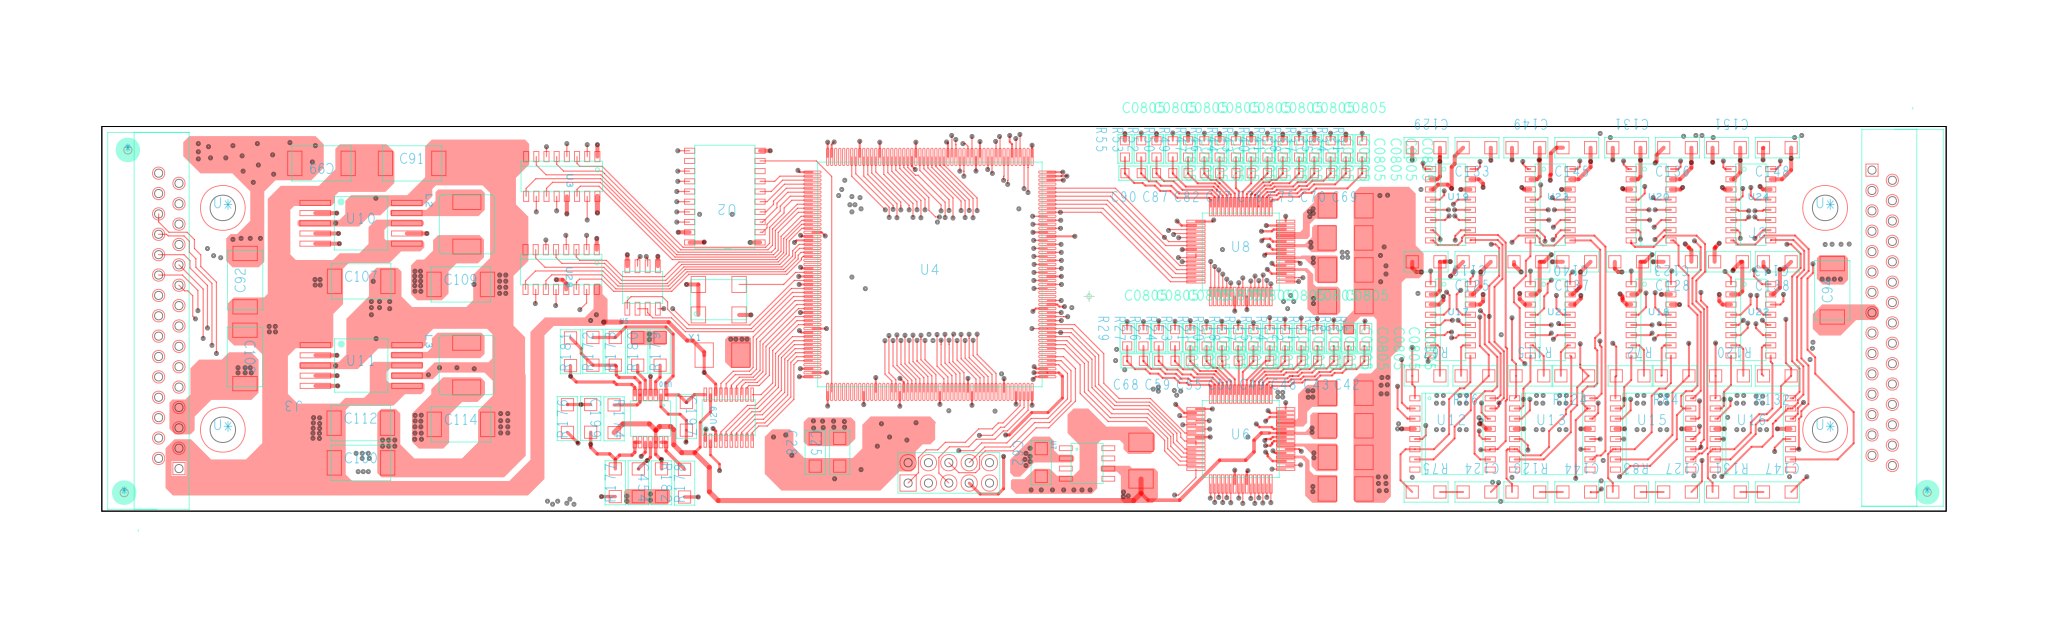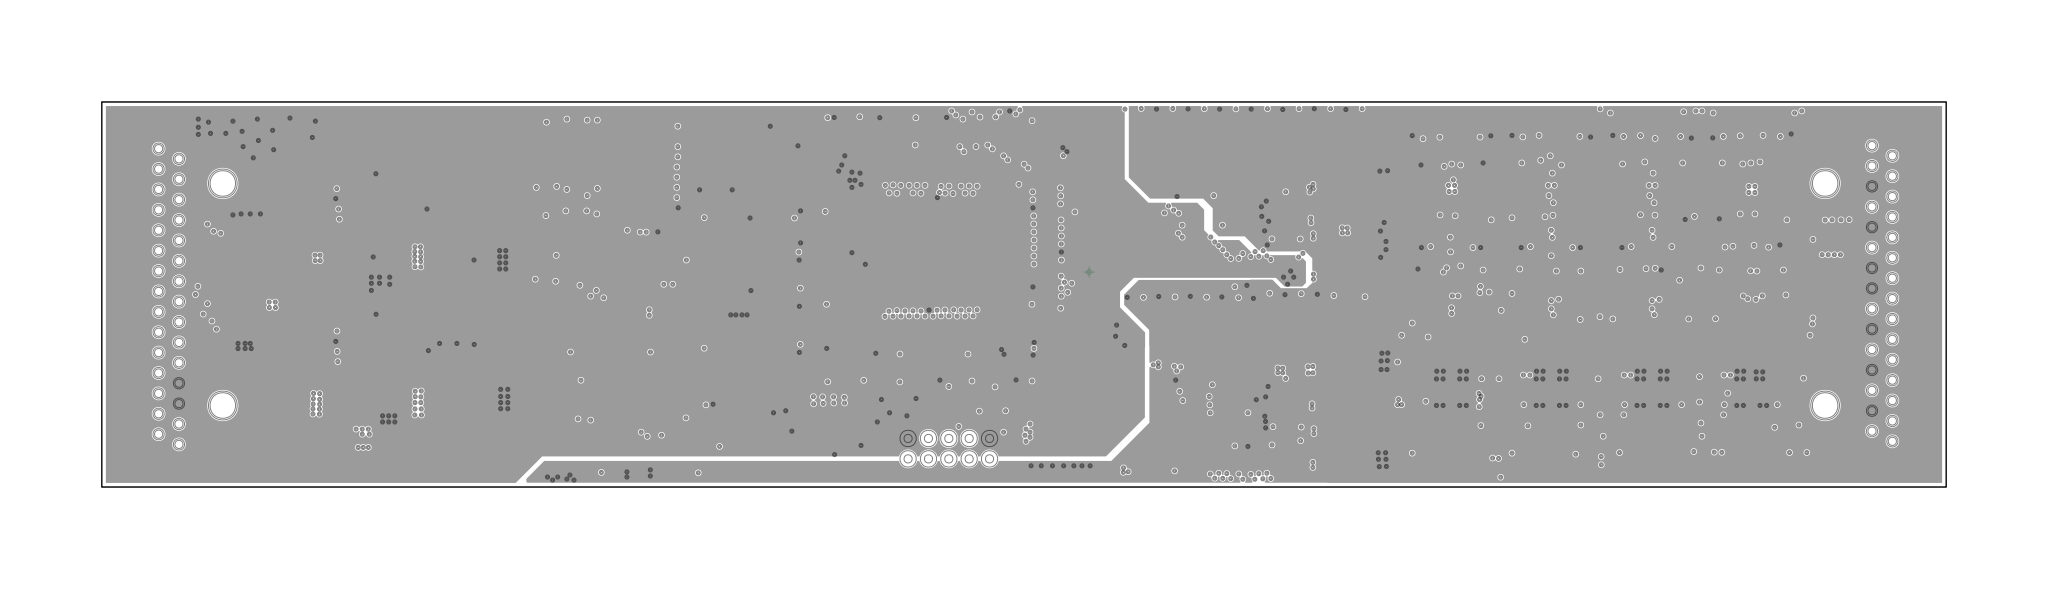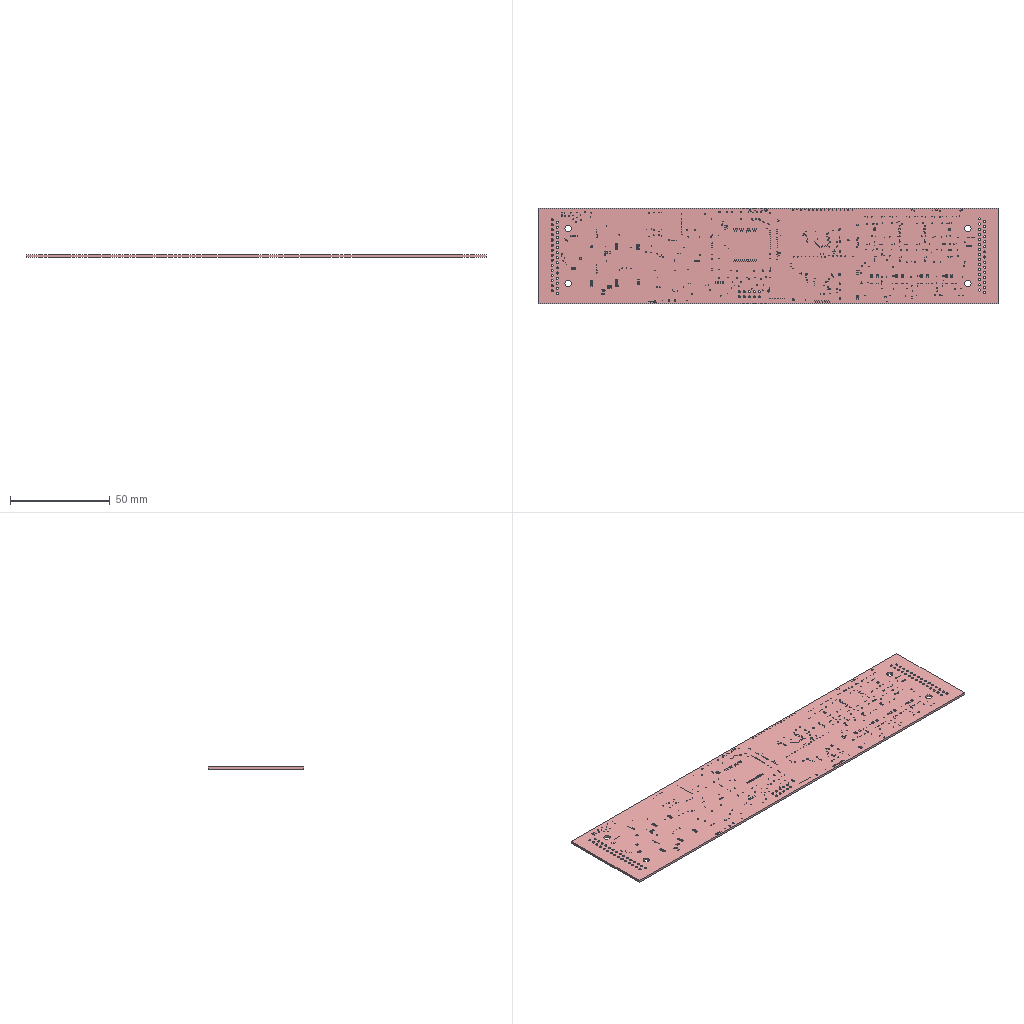Circuit board layout | Cadence Allegro | box 230.1 x 48 x 1.1 mm
Layer stack:
# Cadence Allegro layer stack of  (unit mm; from the constraint file cross-section; dielectric type: 0 not recorded (Allegro does not mark core vs prepreg), 3 surface material)
index,name,kind,layer,copper_thickness_mm,dielectric_type,dielectric_thickness_mm,dielectric_material,dielectric_constant
0,Top Surface,other,,,,,,
1,TOP,copper,TOP,0.0305,,,,
2,Dielectric1,dielectric,,,0,0.2032,FR-4,4.5
3,GND2,copper,GND2,0.0305,,,,
4,Dielectric2,dielectric,,,0,0.2032,FR-4,4.5
5,L3,copper,L3,0.0305,,,,
6,Dielectric3,dielectric,,,0,0.2032,FR-4,4.5
7,VCC4,copper,VCC4,0.0305,,,,
8,Dielectric4,dielectric,,,0,0.2032,FR-4,4.5
9,GND5,copper,GND5,0.0305,,,,
10,Dielectric5,dielectric,,,0,0.2032,FR-4,4.5
11,BOTTOM,copper,BOTTOM,0.0305,,,,
12,Bottom Surface,other,,,,,,
# drill layer pairs: low layer,high layer
drill_pair,TOP,BOTTOM
Part placement:
REFDES,COMP_VALUE,SYM_NAME,SYM_X,SYM_Y,SYM_ROTATE,SYM_MIRROR
C1,0.1uF,1206,57.000,79.000,180.000,YES
C2,0.1uF,1206,-1295.000,-350.000,180.000,YES
C3,0.1uF,1206,56.000,295.000,180.000,YES
C4,0.1uF,1206,-2483.000,577.000,0.000,YES
C5,0.1uF,1206,-2483.000,467.000,0.000,YES
C6,0.1uF,1206,-2483.000,682.000,0.000,YES
C7,0.1uF,1206,-215.000,-470.000,180.000,YES
C8,0.1uF,1206,-1125.000,630.000,90.000,YES
C9,0.1uF,1206,-250.000,575.000,0.000,YES
C10,0.1uF,1206,-455.000,60.000,270.000,YES
C11,0.1uF,1206,-210.000,690.000,180.000,YES
C12,0.1uF,1206,-450.000,-260.000,90.000,YES
C13,0.1uF,1206,-1350.000,-470.000,0.000,YES
C14,0.1uF,1206,-205.000,35.000,270.000,YES
C15,0.1uF,1206,56.000,187.000,180.000,YES
C16,0.1uF,1206,-1285.000,630.000,90.000,YES
C17,0.1uF,1206,-345.000,59.000,270.000,YES
C18,0.1uF,1206,-1961.000,335.000,270.000,YES
C19,0.1uF,1206,-1806.000,335.000,270.000,YES
C20,0.1uF,1206,-345.000,305.000,90.000,YES
C21,0.1uF,1206,-455.000,305.000,90.000,YES
C22,0.1uF,1206,-1100.000,-90.000,270.000,YES
C23,0.1uF,1206,-1210.000,-90.000,270.000,YES
C24,0.1uF,1206,-1250.000,365.000,270.000,YES
C25,0.1uF,1206,-1225.000,-765.000,270.000,NO
C26,0.1uF,1206,-525.000,-465.000,180.000,YES
C27,0.1uF,1206,-1000.000,-470.000,0.000,YES
C28,0.1uF,1206,-1345.000,-765.000,270.000,NO
C29,0.1uF,1206,-1345.000,-765.000,90.000,YES
C30,0.1uF,1206,-1360.000,365.000,270.000,YES
C31,0.1uF,1206,-940.000,695.000,0.000,YES
C32,0.1uF,1206,-200.000,405.000,270.000,YES
C33,0.1uF,1206,-480.000,695.000,180.000,YES
C34,0.1uF,1206,-1295.000,100.000,180.000,YES
C35,0.1uF,1206,-1355.000,-150.000,90.000,YES
C36,0.1uF,1206,-1225.000,-765.000,90.000,YES
C37,1uF,1206,-1849.000,-86.000,180.000,YES
C38,0.1uF,1206,-1849.000,24.000,180.000,YES
C39,0.1uF,1206,-325.000,-305.000,270.000,YES
C40,0.01uF,1206,-205.000,-305.000,270.000,YES
C41,0.1uF,1206,-2198.000,149.000,180.000,YES
C42,DNP,0805,1312.000,-316.000,0.000,NO
C43,DNP,0805,1162.000,-316.000,0.000,NO
C44,0.1uF,1206,1220.000,-945.000,0.000,YES
C45,10uF,6032,1160.000,-945.000,0.000,NO
C46,10uF,6032,1160.000,-790.000,0.000,NO
C47,0.1uF,1206,1220.000,-790.000,0.000,YES
C48,DNP,0805,1002.000,-316.000,0.000,NO
C49,DNP,0805,847.000,-316.000,0.000,NO
C50,DNP,0805,692.000,-316.000,0.000,NO
C51,0.01uF,0805,950.000,-610.000,0.000,YES
C52,0.01uF,0805,950.000,-715.000,0.000,YES
C53,0.01uF,0805,950.000,-800.000,0.000,YES
C54,0.01uF,0805,520.000,-530.000,0.000,YES
C55,DNP,0805,537.000,-316.000,0.000,NO
C56,10uF,6032,1360.000,-635.000,180.000,NO
C57,10uF,6032,1160.000,-475.000,0.000,NO
C58,0.1uF,1206,645.000,-930.000,0.000,YES
C59,DNP,0805,382.000,-316.000,0.000,NO
C60,0.01uF,0805,-235.000,-785.000,90.000,YES
C61,1nF,0805,840.000,-930.000,180.000,YES
C62,0.1uF,1206,-235.000,-815.000,270.000,NO
C63,10uF,6032,255.000,-906.000,90.000,NO
C64,0.1uF,1206,1210.000,-635.000,0.000,YES
C65,0.1uF,1206,1220.000,-475.000,180.000,YES
C66,0.01uF,0805,55.000,-845.000,0.000,YES
C67,0.1uF,1206,255.000,-826.000,270.000,YES
C68,DNP,0805,227.000,-316.000,0.000,NO
C69,DNP,0805,1301.000,605.000,0.000,NO
C70,DNP,0805,1146.000,605.000,0.000,NO
C71,0.1uF,1206,1220.000,-25.000,0.000,YES
C72,10uF,6032,1160.000,-25.000,0.000,NO
C73,10uF,6032,1160.000,130.000,0.000,NO
C74,0.1uF,1206,1220.000,130.000,0.000,YES
C75,DNP,0805,991.000,605.000,0.000,NO
C76,DNP,0805,836.000,605.000,0.000,NO
C77,DNP,0805,681.000,605.000,0.000,NO
C78,0.01uF,0805,950.000,120.000,0.000,YES
C79,0.01uF,0805,950.000,205.000,0.000,YES
C80,0.01uF,0805,950.000,310.000,0.000,YES
C81,0.01uF,0805,525.000,380.000,0.000,YES
C82,DNP,0805,526.000,605.000,0.000,NO
C83,10uF,6032,1359.000,287.000,180.000,NO
C84,10uF,6032,1160.000,445.000,0.000,NO
C85,0.1uF,1206,650.000,0.000,0.000,YES
C86,1nF,0805,850.000,0.000,180.000,YES
C87,DNP,0805,371.000,605.000,0.000,NO
C88,0.1uF,1206,1210.000,285.000,0.000,YES
C89,0.1uF,1206,1220.000,445.000,180.000,YES
C90,DNP,0805,216.000,605.000,0.000,NO
C91,10uF/50V,7343,-3325.000,653.000,0.000,NO
C92,10uF/50V,7343,-4145.000,80.000,90.000,NO
C93,10uF/50V,7343,3650.000,25.000,90.000,YES
C94,10uF/50V,7343,3650.000,30.000,90.000,NO
C99,10uF/50V,7343,-3770.000,653.000,180.000,NO
C100,10uF/50V,7343,-3576.000,-817.000,0.000,NO
C101,10uF/50V,7343,-4147.000,-298.000,90.000,YES
C102,10uF/50V,7343,-4146.000,-297.000,270.000,NO
C107,10uF/50V,7343,-3575.000,74.000,0.000,NO
C108,0.1uF,1206,-3640.000,74.000,0.000,YES
C109,10uF/50V,7343,-3086.000,59.000,0.000,NO
C110,0.1uF,1206,-3146.000,59.000,0.000,YES
C111,1nF,1206,-3571.000,439.000,0.000,YES
C112,10uF/50V,7343,-3577.000,-622.000,0.000,NO
C113,0.1uF,1206,-3637.000,-622.000,0.000,YES
C114,10uF/50V,7343,-3085.000,-628.000,0.000,NO
C115,0.1uF,1206,-3150.000,-628.000,0.000,YES
C116,1nF,1206,-3570.000,-259.000,0.000,YES
C117,0.01uF,1206,1905.000,-570.000,0.000,YES
C118,0.01uF,1206,2890.000,-570.000,0.000,YES
C119,0.01uF,1206,1655.000,170.000,180.000,NO
C120,0.01uF,1206,1655.000,-570.000,180.000,YES
C121,0.01uF,1206,2640.000,-570.000,180.000,YES
C122,100nF,1206,1905.000,-310.000,0.000,YES
C123,0.01uF,1206,2650.000,170.000,180.000,NO
C124,100nF,1206,1905.000,-960.000,180.000,NO
C125,0.01uF,1206,1905.000,170.000,0.000,NO
C126,100nF,1206,2890.000,-310.000,0.000,YES
C127,100nF,1206,2890.000,-960.000,180.000,NO
C128,0.01uF,1206,2890.000,170.000,0.000,NO
C129,0.01uF,1206,1655.000,730.000,180.000,NO
C130,100nF,1206,1655.000,-830.000,180.000,YES
C131,0.01uF,1206,2640.000,730.000,180.000,NO
C132,100nF,1206,1905.000,-960.000,0.000,YES
C133,0.01uF,1206,1905.000,730.000,0.000,NO
C134,100nF,1206,2640.000,-830.000,180.000,YES
C135,100nF,1206,2890.000,-960.000,0.000,YES
C136,0.01uF,1206,2890.000,730.000,0.000,NO
C137,0.01uF,1206,2395.000,170.000,0.000,NO
C138,0.01uF,1206,3380.000,170.000,0.000,NO
C139,0.01uF,1206,2145.000,-570.000,180.000,YES
C140,0.01uF,1206,2155.000,170.000,180.000,NO
C141,0.01uF,1206,3130.000,-570.000,180.000,YES
C142,100nF,1206,2395.000,-310.000,0.000,YES
C143,0.01uF,1206,3140.000,170.000,180.000,NO
C144,100nF,1206,2395.000,-960.000,180.000,NO
C145,0.01uF,1206,2395.000,730.000,0.000,NO
C146,100nF,1206,3355.000,-310.000,0.000,YES
C147,100nF,1206,3380.000,-960.000,180.000,NO
C148,0.01uF,1206,3380.000,730.000,0.000,NO
C149,0.01uF,1206,2145.000,730.000,180.000,NO
C150,100nF,1206,2145.000,-830.000,180.000,YES
C151,0.01uF,1206,3130.000,730.000,180.000,NO
C152,100nF,1206,2395.000,-960.000,0.000,YES
C153,0.01uF,1206,2395.000,-570.000,0.000,YES
C154,100nF,1206,3130.000,-830.000,180.000,YES
C155,100nF,1206,3355.000,-960.000,0.000,YES
C156,0.01uF,1206,3355.000,-570.000,0.000,YES
C187,0.1uF,1206,-2488.000,-23.000,0.000,YES
C188,0.1uF,1206,-2488.000,92.000,0.000,YES
C189,0.1uF,1206,-2498.000,202.000,0.000,YES
C192,0.01uF,1206,-2220.540,-453.000,0.000,YES
C197,100nF,1206,-1978.000,-588.540,270.000,NO
C198,100nF,1206,-2447.000,-598.540,90.000,YES
C199,100nF,1206,-2448.000,-598.540,270.000,NO
C200,0.01uF,1206,-2100.000,-914.540,90.000,YES
C201,0.01uF,1206,-1988.000,-914.460,270.000,YES
C202,0.1uF,1206,-1820.000,-289.000,0.000,YES
C451,10uF,6032,-1900.460,-288.000,0.000,NO
C452,0.01uF,1206,-2214.000,-914.540,90.000,YES
C453,0.01uF,1206,-2108.000,-269.460,270.000,YES
C454,0.01uF,1206,-2214.000,-914.540,270.000,NO
C455,0.01uF,1206,-2560.000,-600.000,270.000,YES
J1,HEADER 2X5,HDR5X2_6240_ST,-889.000,-916.000,0.000,NO
J2,J21,GH_30M,3345.000,-730.000,0.000,NO
J3,J21,GH_30M,-3970.000,505.000,180.000,NO
L2,10uH,IND-SPD0735,-3056.000,354.000,270.000,NO
L3,10uH,IND-SPD0735,-3057.000,-337.000,270.000,NO
R2,47K,0805,-462.000,-642.000,90.000,YES
R3,47K,0805,-689.000,-642.000,90.000,YES
R4,\,1206,-2199.000,260.000,180.000,YES
R5,0,0805,1353.000,-203.000,270.000,NO
R6,DNP,0805,1349.000,-170.000,0.000,YES
R7,5K,0805,685.000,-690.000,0.000,YES
R8,0,0805,1276.000,-203.000,270.000,NO
R9,0,0805,1201.000,-203.000,270.000,NO
R10,DNP,0805,1194.000,-170.000,0.000,YES
R11,0,0805,1121.000,-203.000,270.000,NO
R12,0,0805,1042.000,-203.000,270.000,NO
R13,DNP,0805,1035.000,-170.000,0.000,YES
R14,0,0805,962.000,-203.000,270.000,NO
R15,0,0805,887.000,-203.000,270.000,NO
R16,DNP,0805,880.000,-170.000,0.000,YES
R17,0,0805,807.000,-203.000,270.000,NO
R18,0,0805,732.000,-203.000,270.000,NO
R19,DNP,0805,725.000,-170.000,0.000,YES
R20,0,0805,652.000,-203.000,270.000,NO
R21,0,0805,577.000,-203.000,270.000,NO
R22,DNP,0805,570.000,-170.000,0.000,YES
R23,0,0805,497.000,-203.000,270.000,NO
R24,0,0805,422.000,-203.000,270.000,NO
R25,DNP,0805,415.000,-170.000,0.000,YES
R26,0,0805,342.000,-203.000,270.000,NO
R27,0,0805,267.000,-203.000,270.000,NO
R28,DNP,0805,260.000,-170.000,0.000,YES
R29,0,0805,187.000,-203.000,270.000,NO
R30,0,0805,80.000,720.000,0.000,YES
R31,0,0805,1341.000,724.000,270.000,NO
R32,DNP,0805,1345.000,750.000,0.000,YES
R33,5K,0805,565.000,230.000,0.000,YES
R34,0,0805,1261.000,724.000,270.000,NO
R35,0,0805,1186.000,724.000,270.000,NO
R36,DNP,0805,1190.000,750.000,0.000,YES
R37,0,0805,1106.000,724.000,270.000,NO
R38,0,0805,1031.000,724.000,270.000,NO
R39,DNP,0805,1035.000,750.000,0.000,YES
R40,0,0805,876.000,724.000,270.000,NO
R41,0,0805,951.000,724.000,270.000,NO
R42,DNP,0805,880.000,750.000,0.000,YES
R43,0,0805,796.000,724.000,270.000,NO
R44,0,0805,721.000,724.000,270.000,NO
R45,DNP,0805,725.000,750.000,0.000,YES
R46,0,0805,641.000,724.000,270.000,NO
R47,0,0805,566.000,724.000,270.000,NO
R48,DNP,0805,570.000,750.000,0.000,YES
R49,0,0805,486.000,724.000,270.000,NO
R50,0,0805,411.000,724.000,270.000,NO
R51,DNP,0805,415.000,750.000,0.000,YES
R52,0,0805,331.000,724.000,270.000,NO
R53,0,0805,256.000,724.000,270.000,NO
R54,DNP,0805,260.000,750.000,0.000,YES
R55,0,0805,176.000,724.000,270.000,NO
R56,0,0805,-3665.000,-815.000,180.000,YES
R60,630K,0805,-3571.000,259.000,0.000,YES
R61,320K,0805,-3571.000,344.000,0.000,YES
R62,100K,0805,-3796.000,299.000,270.000,YES
R63,140K,0805,-3569.000,-442.000,0.000,YES
R64,320K,0805,-3571.000,-355.000,0.000,YES
R65,60K,0805,-3815.000,-400.000,270.000,YES
R66,3K,1206,1655.000,-440.000,180.000,YES
R67,60.4K,1206,1655.000,-390.000,180.000,NO
R68,30K,1206,1655.000,-180.000,0.000,YES
R69,3K,1206,2640.000,-440.000,180.000,YES
R70,15K,1206,1655.000,-50.000,0.000,YES
R71,7.5K,1206,1655.000,80.000,0.000,YES
R72,60.4K,1206,2657.000,-390.000,180.000,NO
R73,10K,1206,1655.000,-310.000,0.000,YES
R74,30K,1206,2640.000,-180.000,0.000,YES
R75,10K,1206,1655.000,-960.000,180.000,NO
R76,60.4K,1206,1895.000,-390.000,0.000,NO
R77,15K,1206,2640.000,-50.000,0.000,YES
R78,30K,1206,1905.000,-180.000,180.000,YES
R79,7.5K,1206,2640.000,80.000,0.000,YES
R80,15K,1206,1905.000,-50.000,180.000,YES
R81,10K,1206,2640.000,-310.000,0.000,YES
R82,7.5K,1206,1905.000,80.000,180.000,YES
R83,10K,1206,2640.000,-960.000,180.000,NO
R84,60.4K,1206,2878.000,-390.000,0.000,NO
R85,30K,1206,2890.000,-180.000,180.000,YES
R86,3K,1206,1655.000,-700.000,180.000,YES
R87,15K,1206,2890.000,-50.000,180.000,YES
R88,7.5K,1206,2880.000,80.000,180.000,YES
R89,3K,1206,2640.000,-700.000,180.000,YES
R90,3K,1206,1905.000,-700.000,0.000,YES
R91,60.4K,1206,1655.000,210.000,0.000,YES
R92,30K,1206,1655.000,340.000,0.000,YES
R93,3K,1206,2890.000,-700.000,0.000,YES
R94,15K,1206,1655.000,470.000,0.000,YES
R95,7.5K,1206,1655.000,600.000,0.000,YES
R96,60.4K,1206,2640.000,210.000,0.000,YES
R97,10K,1206,1905.000,-830.000,180.000,YES
R98,30K,1206,2640.000,340.000,0.000,YES
R99,10K,1206,1655.000,-960.000,0.000,YES
R100,60.4K,1206,1905.000,210.000,180.000,YES
R101,15K,1206,2640.000,470.000,0.000,YES
R102,30K,1206,1905.000,340.000,180.000,YES
R103,7.5K,1206,2640.000,600.000,0.000,YES
R104,15K,1206,1905.000,470.000,180.000,YES
R105,10K,1206,2890.000,-830.000,180.000,YES
R106,7.5K,1206,1905.000,600.000,180.000,YES
R107,10K,1206,2640.000,-960.000,0.000,YES
R108,60.4K,1206,2890.000,210.000,180.000,YES
R109,30K,1206,2890.000,340.000,180.000,YES
R110,3K,1206,1905.000,-440.000,0.000,YES
R111,15K,1206,2890.000,470.000,180.000,YES
R112,7.5K,1206,2890.000,600.000,180.000,YES
R113,3K,1206,2890.000,-440.000,0.000,YES
R114,3K,1206,2145.000,-440.000,180.000,YES
R115,60.4K,1206,2165.000,-390.000,180.000,NO
R116,30K,1206,2145.000,-180.000,0.000,YES
R117,3K,1206,3130.000,-440.000,180.000,YES
R118,15K,1206,2145.000,-50.000,0.000,YES
R119,7.5K,1206,2145.000,80.000,0.000,YES
R120,60.4K,1206,3145.000,-390.000,180.000,NO
R121,10K,1206,2145.000,-310.000,0.000,YES
R122,30K,1206,3130.000,-180.000,0.000,YES
R123,10K,1206,2145.000,-960.000,180.000,NO
R124,60.4K,1206,2385.000,-390.000,0.000,NO
R125,15K,1206,3130.000,-50.000,0.000,YES
R126,30K,1206,2395.000,-180.000,180.000,YES
R127,7.5K,1206,3135.000,80.000,0.000,YES
R128,15K,1206,2395.000,-50.000,180.000,YES
R129,10K,1206,3130.000,-310.000,0.000,YES
R130,7.5K,1206,2395.000,80.000,180.000,YES
R131,10K,1206,3130.000,-960.000,180.000,NO
R132,60.4K,1206,3380.000,-390.000,0.000,NO
R133,30K,1206,3355.000,-180.000,180.000,YES
R134,3K,1206,2145.000,-700.000,180.000,YES
R135,15K,1206,3355.000,-50.000,180.000,YES
R136,7.5K,1206,3355.000,80.000,180.000,YES
R137,3K,1206,3130.000,-700.000,180.000,YES
R138,3K,1206,2395.000,-700.000,0.000,YES
R139,60.4K,1206,2145.000,210.000,0.000,YES
R140,30K,1206,2145.000,340.000,0.000,YES
R141,3K,1206,3355.000,-700.000,0.000,YES
R142,15K,1206,2145.000,470.000,0.000,YES
R143,7.5K,1206,2145.000,600.000,0.000,YES
R144,60.4K,1206,3130.000,210.000,0.000,YES
R145,10K,1206,2395.000,-830.000,180.000,YES
R146,30K,1206,3130.000,340.000,0.000,YES
R147,10K,1206,2145.000,-960.000,0.000,YES
R148,60.4K,1206,2395.000,210.000,180.000,YES
R149,15K,1206,3130.000,470.000,0.000,YES
R150,30K,1206,2395.000,340.000,180.000,YES
R151,7.5K,1206,3130.000,600.000,0.000,YES
R152,15K,1206,2395.000,470.000,180.000,YES
R153,10K,1206,3355.000,-830.000,180.000,YES
R154,7.5K,1206,2395.000,600.000,180.000,YES
R155,10K,1206,3130.000,-960.000,0.000,YES
R156,60.4K,1206,3355.000,210.000,180.000,YES
R157,30K,1206,3355.000,340.000,180.000,YES
R158,3K,1206,2395.000,-440.000,0.000,YES
R159,15K,1206,3355.000,470.000,180.000,YES
R160,7.5K,1206,3355.000,600.000,180.000,YES
R161,3K,1206,3355.000,-440.000,0.000,YES
R172,10K,1206,-2437.000,-269.460,90.000,NO
R173,10K,1206,-2327.000,-269.460,90.000,NO
R174,10K,1206,-2333.000,-600.540,270.000,NO
R175,10K,1206,-2480.540,-338.000,0.000,YES
R176,10K,1206,-2562.000,-599.460,90.000,NO
R177,10K,1206,-2327.000,-914.460,90.000,NO
R178,2K,1206,-1987.000,-916.460,90.000,NO
R179,10K,1206,-2107.000,-269.460,90.000,NO
R180,10K,1206,-2217.000,-269.460,90.000,NO
R181,20K,1206,-2547.000,-271.460,90.000,NO
R182,10K,1206,-2100.000,-914.540,270.000,NO
U1,IS61WV102416,TSSOP48W,-776.406,105.882,90.000,YES
U2,74HC244,SOIC20,-1616.000,265.000,180.000,NO
U3,MC14504B,SOIC16,-2590.000,589.000,270.000,NO
U4,A3P1000,PQFP208,-782.000,108.000,0.000,NO
U5,SN65HVD08D,SO-8,-2193.000,44.000,0.000,NO
U6,AD7608-1,TQFP64,745.000,-700.000,0.000,NO
U7,ADR425,SO-8,-10.000,-820.000,270.000,NO
U8,AD7608-1,TQFP64,745.000,220.000,0.000,NO
U10,TPS62000,CFP10,-3576.000,359.000,0.000,NO
U11,TPS62000,CFP10,-3575.000,-339.000,0.000,NO
U12,OP470,SOIC16W,1785.000,-675.000,0.000,NO
U13,OP470,SOIC16W,2275.000,-675.000,0.000,NO
U15,OP470,SOIC16W,2770.000,-675.000,0.000,NO
U16,OP470,SOIC16W,3260.000,-675.000,0.000,NO
U17,DG406,SO-16,1775.000,-115.000,0.000,NO
U18,DG406,SO-16,2760.000,-115.000,0.000,NO
U19,DG406,SO-16,1775.000,450.000,0.000,NO
U20,DG406,SO-16,2760.000,450.000,0.000,NO
U21,DG406,SO-16,2265.000,-115.000,0.000,NO
U22,DG406,SO-16,3250.000,-115.000,0.000,NO
U23,DG406,SO-16,2265.000,450.000,0.000,NO
U24,DG406,SO-16,3250.000,450.000,0.000,NO
U28,MC14504B,SOIC16,-2593.000,132.000,270.000,NO
U29,AD7945,TSSOP20,-1770.000,-595.000,90.000,NO
U30,OP471AY,TSSOP-14,-2154.270,-599.540,180.000,NO
Y1,10MHZ,OSC-5X7MM,-1819.000,-16.000,0.000,NO
Pad and via stacks:
# Allegro (Cadence) via spans and padstacks; design units: ("mils" 3 1000)
# via spans: padstack,start_layer,end_layer,net_example,count
VIA_20D10,ETCH/TOP,ETCH/BOTTOM,DATA_OUT_B5,812
# Allegro padstack definitions: name,start_layer,end_layer,drill,plating,holeType,type
SMDSQR_60,"ETCH/TOP","ETCH/TOP",0.0,"PLATED","none","smd"
SMD65REC13,"ETCH/TOP","ETCH/TOP",0.0,"PLATED","none","smd"
SMD-R0-45X1-4_MM,"ETCH/TOP","ETCH/TOP",0.0,"PLATED","none","smd"
SMD50_25,"ETCH/TOP","ETCH/TOP",0.0,"PLATED","none","smd"
SMDREC_70X120,"ETCH/TOP","ETCH/TOP",0.0,"PLATED","none","smd"
SMD40_45,"ETCH/TOP","ETCH/TOP",0.0,"PLATED","none","smd"
SMDREC_90X120,"ETCH/TOP","ETCH/TOP",0.0,"PLATED","none","smd"
PAD60CIR40D,"ETCH/TOP","ETCH/BOTTOM",40.0,"PLATED","circle_drill","through"
PAD60SQ40D,"ETCH/TOP","ETCH/BOTTOM",40.0,"PLATED","circle_drill","through"
SMD70REC10,"ETCH/TOP","ETCH/TOP",0.0,"PLATED","none","smd"
SMD-R0-6X1-6_MM,"ETCH/TOP","ETCH/TOP",0.0,"PLATED","none","smd"
SMD90_15,"ETCH/TOP","ETCH/TOP",0.0,"PLATED","none","smd"
SMD25_50,"ETCH/TOP","ETCH/TOP",0.0,"PLATED","none","smd"
PAD49,"ETCH/TOP","ETCH/TOP",0.0,"PLATED","none","smd"
SMD-R1-85X3-5_MM,"ETCH/TOP","ETCH/TOP",0.0,"PLATED","none","smd"
SMD160_25,"ETCH/TOP","ETCH/TOP",0.0,"PLATED","none","smd"
PAD80SQ40D,"ETCH/TOP","ETCH/BOTTOM",40.0,"PLATED","circle_drill","through"
CIR_80D40,"ETCH/TOP","ETCH/BOTTOM",40.0,"PLATED","circle_drill","through"
SMD-R1-8X2_MM,"ETCH/TOP","ETCH/TOP",0.0,"PLATED","none","smd"
CIR_220D125,"ETCH/TOP","ETCH/BOTTOM",125.0,"PLATED","circle_drill","through"
C40-TEST118,"ETCH/TOP","ETCH/TOP",0.0,"PLATED","none","smd"
VIA_20D10,"ETCH/TOP","ETCH/BOTTOM",10.0,"PLATED","circle_drill","through"
Design rules, without the lines most boards share, first 14 of 26 lines:
# Cadence Allegro design rules of  (from the Constraint Manager export constraints.dcfx, design unit mil; typed fields in mm)
# columns: name | kind | enabled | priority | scope1 | scope2 | descriptor | typed fields (field=value)
# Allegro precedence (priority 1 wins): 1 Region class-to-class, 2 Region class, 3 Region, 4 class-to-class, 5 DiffPair/Bus/NetGroup override, 6 NetClass, 7 constraint set (CSet) default
# per-layer values are written LAYER=value in the descriptor and LAYER:mm in the typed field; a maximum of 0 means no limit set
# --- net classes (and buses / net groups) ---
# (no net classes defined: every net uses the default constraint sets)
# --- track widths, neck and differential-pair gap (physical constraint sets) ---
DEFAULT | PhysicalCSet | enabled | 7 | Design default | All | Physical Constraint (Min Line Width=6mil) (Max Line Width=100mil) (Min Neck Width=8mil) (Max Neck Length=100000mil) (DiffPair Primary Gap=6mil) (DiffPair Neck Gap=0mil) (DiffPair Min Space=0mil) (DiffPair Coupled +Tol=0mil) (DiffPair Coupled -Tol=0mil) (Min BB Via Stagger=5mil) (Max BB Via Stagger=0mil) (T-junctions=ANYWHERE) (Pad-pad direct connect=ALL_ALLOWED) (Allowed vias=VIA_20D10) | min_line_width=0.1524 min_neck_width=0.2032 min_bvia_stagger=0.127 max_bvia_stagger=0 ts_allowed=ANYWHERE diffp_primary_gap=0.1524 diffp_neck_gap=0 max_line_width=2.54 maximum_neck_length=2540 pad_pad_direct_connect=ALL_ALLOWED allow_on_etch_subclass=TRUE diffp_coupled_plus=0 diffp_coupled_minus=0 diffp_min_space=0 vias=VIA_20D10
# --- clearances: line / pad / via / shape / hole (spacing constraint sets) ---
DEFAULT | SpacingCSet | enabled | 7 | Design default | All | Clearance Constraint (Line-Line=6mil) (Line-SMD Pad=6mil) (Line-Thru Pin=6mil) (Line-Via=6mil) (Line-Shape=6mil) (SMD Pad-SMD Pad=6mil) (Thru Pin-Thru Pin=6mil) (Thru Pin-SMD Pad=6mil) (SMD Pad-Via=6mil) (Thru Pin-Via=6mil) (Via-Via=6mil) (Shape-SMD Pad=6mil) (Shape-Thru Pin=6mil) (Shape-Via=6mil) (Shape-Shape=6mil) (Hole-Hole=6mil) (Hole-Line=6mil) (Hole-Shape=6mil) (BB Via-BB Via=6mil) (uVia-uVia=5mil) | thrupin_to_thrupin_spacing=0.1524 thrupin_to_smdpin_spacing=0.1524 thrupin_to_thruvia_spacing=0.1524 line_to_thrupin_spacing=0.1524 thrupin_to_shape_spacing=0.1524 smdpin_to_smdpin_spacing=0.1524 smdpin_to_thruvia_spacing=0.1524 line_to_smdpin_spacing=0.1524 shape_to_smdpin_spacing=0.1524 thruvia_to_thruvia_spacing=0.1524 line_to_thruvia_spacing=0.1524 shape_to_thruvia_spacing=0.1524 line_to_line_spacing=0.1524 line_to_shape_spacing=0.1524 shape_to_shape_spacing=0.1524 bbv_to_bbv_spacing=0.1524 bbv_to_thrupin_spacing=0.1524 bbv_to_smdpin_spacing=0.1524 bbv_to_thruvia_spacing=0.1524 bbv_to_line_spacing=0.1524 bbv_to_shape_spacing=0.1524 bbv_to_testpin_spacing=0.1524 bbv_to_testvia_spacing=0.1524 testpin_to_testpin_spacing=0.1524 testpin_to_thrupin_spacing=0.1524 smdpin_to_testpin_spacing=0.1524 testpin_to_thruvia_spacing=0.1524 testpin_to_testvia_spacing=0.1524 line_to_testpin_spacing=0.1524 shape_to_testpin_spacing=0.1524 testvia_to_testvia_spacing=0.1524 testvia_to_thrupin_spacing=0.1524 smdpin_to_testvia_spacing=0.1524 testvia_to_thruvia_spacing=0.1524 line_to_testvia_spacing=0.1524 shape_to_testvia_spacing=0.1524 bondpad_to_bondpad_spacing=0.1524 thrupin_to_bondpad_spacing=0.1524 smdpin_to_bondpad_spacing=0.1524 bondpad_to_thruvia_spacing=0.1524 bondpad_to_line_spacing=0.1524 bondpad_to_shape_spacing=0.1524 bondpad_to_bbv_spacing=0.1524 bondpad_to_testpin_spacing=0.1524 bondpad_to_testvia_spacing=0.1524 min_bvia_gap=0.254 hole_to_pin_spacing=0.1524 hole_to_via_spacing=0.1524 hole_to_line_spacing=0.1524 hole_to_shape_spacing=0.1524 hole_to_hole_spacing=0.1524 mvia_to_mvia_spacing=0.127 mvia_to_thrupin_spacing=0.2032 mvia_to_smdpin_spacing=0.2032 mvia_to_thruvia_spacing=0.2032 mvia_to_bbv_spacing=0.2032 mvia_to_line_spacing=0.2032 mvia_to_shape_spacing=0.3048 mvia_to_testpin_spacing=0.2032 mvia_to_testvia_spacing=0.2032 bondpad_to_mvia_spacing=0.2032 bondpad_to_bondpad_diffp_spc=0.127
DEFAULT | SameNetSpacingCSet | enabled | 7 | Design default | All | Same-Net Clearance (Line-Line=6mil) (Line-SMD Pad=6mil) (Line-Thru Pin=6mil) (Line-Via=6mil) (Line-Shape=6mil) (SMD Pad-SMD Pad=6mil) (Thru Pin-Thru Pin=6mil) (Thru Pin-SMD Pad=6mil) (SMD Pad-Via=6mil) (Thru Pin-Via=6mil) (Via-Via=6mil) (Shape-SMD Pad=6mil) (Shape-Thru Pin=6mil) (Shape-Via=6mil) (Shape-Shape=5mil) (Hole-Hole=5mil) (Hole-Line=6mil) (Hole-Shape=5mil) (BB Via-BB Via=6mil) (uVia-uVia=5mil) | sn_thrupin_to_thrupin_spacing=0.1524 sn_thrupin_to_smdpin_spacing=0.1524 sn_thrupin_to_thruvia_spacing=0.1524 sn_line_to_thrupin_spacing=0.1524 sn_thrupin_to_shape_spacing=0.1524 sn_smdpin_to_smdpin_spacing=0.1524 sn_smdpin_to_thruvia_spacing=0.1524 sn_line_to_smdpin_spacing=0.1524 sn_shape_to_smdpin_spacing=0.1524 sn_thruvia_to_thruvia_spacing=0.1524 sn_line_to_thruvia_spacing=0.1524 sn_shape_to_thruvia_spacing=0.1524 sn_line_to_line_spacing=0.1524 sn_line_to_shape_spacing=0.1524 sn_shape_to_shape_spacing=0.127 sn_bbv_to_bbv_spacing=0.1524 sn_bbv_to_thrupin_spacing=0.1524 sn_bbv_to_smdpin_spacing=0.1524 sn_bbv_to_thruvia_spacing=0.1524 sn_bbv_to_line_spacing=0.1524 sn_bbv_to_shape_spacing=0.1524 sn_bbv_to_testpin_spacing=0.1524 sn_bbv_to_testvia_spacing=0.1524 sn_testpin_to_testpin_spacing=0.1524 sn_testpin_to_thrupin_spacing=0.1524 sn_smdpin_to_testpin_spacing=0.1524 sn_testpin_to_thruvia_spacing=0.1524 sn_testpin_to_testvia_spacing=0.1524 sn_line_to_testpin_spacing=0.1524 sn_shape_to_testpin_spacing=0.1524 sn_testvia_to_testvia_spacing=0.1524 sn_testvia_to_thrupin_spacing=0.1524 sn_smdpin_to_testvia_spacing=0.1524 sn_testvia_to_thruvia_spacing=0.1524 sn_line_to_testvia_spacing=0.1524 sn_shape_to_testvia_spacing=0.1524 sn_bondpad_to_bondpad_spacing=0.127 sn_thrupin_to_bondpad_spacing=0.1524 sn_smdpin_to_bondpad_spacing=0.1524 sn_bondpad_to_thruvia_spacing=0.1524 sn_bondpad_to_line_spacing=0.1524 sn_bondpad_to_shape_spacing=0.127 sn_bondpad_to_bbv_spacing=0.1524 sn_bondpad_to_testpin_spacing=0.1524 sn_bondpad_to_testvia_spacing=0.1524 same_net=TRUE sn_hole_to_pin_spacing=0.127 sn_hole_to_via_spacing=0.127 sn_hole_to_line_spacing=0.1524 sn_hole_to_shape_spacing=0.127 sn_hole_to_hole_spacing=0.127 sn_mvia_to_mvia_spacing=0.127 sn_mvia_to_thrupin_spacing=0.1524 sn_mvia_to_smdpin_spacing=0.1524 sn_mvia_to_thruvia_spacing=0.1524 sn_mvia_to_bbv_spacing=0.1524 sn_mvia_to_line_spacing=0.1524 sn_mvia_to_shape_spacing=0.127 sn_mvia_to_testpin_spacing=0.1524 sn_mvia_to_testvia_spacing=0.1524 sn_bondpad_to_mvia_spacing=0.127
RGN2 | Region | enabled | 3 | Region RGN2 | All | Region Constraint  |
RGN1 | Region | enabled | 3 | Region RGN1 | All | Region Constraint  |
# --- differential pairs (1) ---